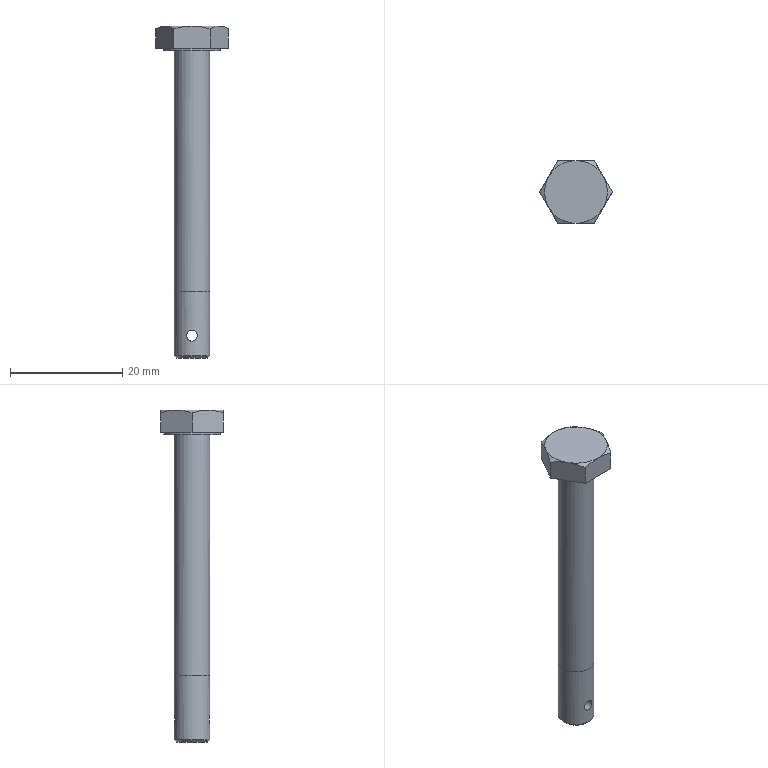Part | NX | features solid 2 | 1 solid | 21 faces | box 12.905 x 11.176 x 59.138 mm | volume 2174 mm3 | plane 10 | cone 7 | cylinder 4 | commonest cylinder face diameters 6.35 x2 1.93 x1 10.109 x1
STEP:
#1=CARTESIAN_POINT('',(0.,-3.175,-56.134));
#2=VERTEX_POINT('',#1);
#3=CARTESIAN_POINT('',(0.7569,-3.102,-55.925));
#4=CARTESIAN_POINT('',(-0.00006064,-3.212,-56.239));
#5=CARTESIAN_POINT('',(-0.7566,-3.102,-55.924));
#6=CARTESIAN_POINT('',(-1.07,-2.986,-55.17));
#7=CARTESIAN_POINT('',(-0.7562,-3.102,-54.412));
#8=CARTESIAN_POINT('',(-0.0005897,-3.212,-54.099));
#9=CARTESIAN_POINT('',(0.7561,-3.102,-54.412));
#10=CARTESIAN_POINT('',(1.07,-2.986,-55.169));
#11=CARTESIAN_POINT('',(0.7569,-3.102,-55.925));
#12=CARTESIAN_POINT('',(-0.00006064,-3.212,-56.239));
#13=CARTESIAN_POINT('',(-0.7566,-3.102,-55.924));
#14=B_SPLINE_CURVE_WITH_KNOTS('',3,(#3,#4,#5,#6,#7,#8,#9,#10,#11,#12,#13),.UNSPECIFIED.,.T.,.F.,(1,1,1,1,1,1,1,1,1,1,1,1,1,1,1),(-0.002276,-0.001518,-0.0007588,0.,0.0007588,0.001518,0.002276,0.003035,0.003794,0.004553,0.005312,0.006071,0.006829,0.007588,0.008347),.UNSPECIFIED.);
#15=EDGE_CURVE('',#2,#2,#14,.T.);
#16=ORIENTED_EDGE('',*,*,#15,.T.);
#17=EDGE_LOOP('',(#16));
#18=FACE_BOUND('',#17,.T.);
#19=CARTESIAN_POINT('',(-3.175,0.,-47.231));
#20=VERTEX_POINT('',#19);
#21=CARTESIAN_POINT('',(-2.488,2.488,-47.231));
#22=CARTESIAN_POINT('',(-3.519,0.,-47.231));
#23=CARTESIAN_POINT('',(-2.488,-2.488,-47.231));
#24=CARTESIAN_POINT('',(0.,-3.519,-47.231));
#25=CARTESIAN_POINT('',(2.488,-2.488,-47.231));
#26=CARTESIAN_POINT('',(3.519,0.,-47.231));
#27=CARTESIAN_POINT('',(2.488,2.488,-47.231));
#28=CARTESIAN_POINT('',(0.,3.519,-47.231));
#29=CARTESIAN_POINT('',(-2.488,2.488,-47.231));
#30=CARTESIAN_POINT('',(-3.519,0.,-47.231));
#31=CARTESIAN_POINT('',(-2.488,-2.488,-47.231));
#32=B_SPLINE_CURVE_WITH_KNOTS('',3,(#21,#22,#23,#24,#25,#26,#27,#28,#29,#30,#31),.UNSPECIFIED.,.T.,.F.,(1,1,1,1,1,1,1,1,1,1,1,1,1,1,1),(-0.375,-0.25,-0.125,0.,0.125,0.25,0.375,0.5,0.625,0.75,0.875,1.,1.125,1.25,1.375),.UNSPECIFIED.);
#33=EDGE_CURVE('',#20,#20,#32,.T.);
#34=ORIENTED_EDGE('',*,*,#33,.F.);
#35=EDGE_LOOP('',(#34));
#36=FACE_BOUND('',#35,.T.);
#37=CARTESIAN_POINT('',(-3.175,0.,-58.757));
#38=VERTEX_POINT('',#37);
#39=CARTESIAN_POINT('',(0.,0.,-58.757));
#40=DIRECTION('',(0.,0.,-1.));
#41=DIRECTION('',(-1.,0.,0.));
#42=AXIS2_PLACEMENT_3D('',#39,#40,#41);
#43=CIRCLE('',#42,3.175);
#44=EDGE_CURVE('',#38,#38,#43,.T.);
#45=ORIENTED_EDGE('',*,*,#44,.F.);
#46=EDGE_LOOP('',(#45));
#47=FACE_BOUND('',#46,.T.);
#48=CARTESIAN_POINT('',(0.,3.175,-56.134));
#49=VERTEX_POINT('',#48);
#50=CARTESIAN_POINT('',(-0.7569,3.102,-55.925));
#51=CARTESIAN_POINT('',(0.00006064,3.212,-56.239));
#52=CARTESIAN_POINT('',(0.7566,3.102,-55.924));
#53=CARTESIAN_POINT('',(1.07,2.986,-55.17));
#54=CARTESIAN_POINT('',(0.7562,3.102,-54.412));
#55=CARTESIAN_POINT('',(0.0005897,3.212,-54.099));
#56=CARTESIAN_POINT('',(-0.7561,3.102,-54.412));
#57=CARTESIAN_POINT('',(-1.07,2.986,-55.169));
#58=CARTESIAN_POINT('',(-0.7569,3.102,-55.925));
#59=CARTESIAN_POINT('',(0.00006064,3.212,-56.239));
#60=CARTESIAN_POINT('',(0.7566,3.102,-55.924));
#61=B_SPLINE_CURVE_WITH_KNOTS('',3,(#50,#51,#52,#53,#54,#55,#56,#57,#58,#59,#60),.UNSPECIFIED.,.T.,.F.,(1,1,1,1,1,1,1,1,1,1,1,1,1,1,1),(-0.002276,-0.001518,-0.0007588,0.,0.0007588,0.001518,0.002276,0.003035,0.003794,0.004553,0.005312,0.006071,0.006829,0.007588,0.008347),.UNSPECIFIED.);
#62=EDGE_CURVE('',#49,#49,#61,.T.);
#63=ORIENTED_EDGE('',*,*,#62,.T.);
#64=EDGE_LOOP('',(#63));
#65=FACE_BOUND('',#64,.T.);
#66=CARTESIAN_POINT('',(0.,0.,0.));
#67=DIRECTION('',(0.,0.,-1.));
#68=DIRECTION('',(-1.,0.,0.));
#69=AXIS2_PLACEMENT_3D('',#66,#67,#68);
#70=CYLINDRICAL_SURFACE('',#69,3.175);
#71=ADVANCED_FACE('',(#18,#36,#47,#65),#70,.T.);
#72=CARTESIAN_POINT('',(-3.175,0.,-4.369));
#73=VERTEX_POINT('',#72);
#74=CARTESIAN_POINT('',(0.,0.,-4.369));
#75=DIRECTION('',(0.,0.,-1.));
#76=DIRECTION('',(-1.,0.,0.));
#77=AXIS2_PLACEMENT_3D('',#74,#75,#76);
#78=CIRCLE('',#77,3.175);
#79=EDGE_CURVE('',#73,#73,#78,.T.);
#80=ORIENTED_EDGE('',*,*,#79,.T.);
#81=EDGE_LOOP('',(#80));
#82=FACE_BOUND('',#81,.T.);
#83=ORIENTED_EDGE('',*,*,#33,.T.);
#84=EDGE_LOOP('',(#83));
#85=FACE_BOUND('',#84,.T.);
#86=CARTESIAN_POINT('',(0.,0.,0.));
#87=DIRECTION('',(0.,0.,-1.));
#88=DIRECTION('',(-1.,0.,0.));
#89=AXIS2_PLACEMENT_3D('',#86,#87,#88);
#90=CYLINDRICAL_SURFACE('',#89,3.175);
#91=ADVANCED_FACE('',(#82,#85),#90,.T.);
#92=CARTESIAN_POINT('',(-6.452,0.,-3.962));
#93=VERTEX_POINT('',#92);
#94=CARTESIAN_POINT('',(-3.226,5.588,-3.962));
#95=VERTEX_POINT('',#94);
#96=CARTESIAN_POINT('',(-3.576,4.983,-3.962));
#97=DIRECTION('',(0.5,0.866,0.));
#98=VECTOR('',#97,1000.);
#99=LINE('',#96,#98);
#100=EDGE_CURVE('',#93,#95,#99,.T.);
#101=ORIENTED_EDGE('',*,*,#100,.T.);
#102=CARTESIAN_POINT('',(3.226,5.588,-3.962));
#103=VERTEX_POINT('',#102);
#104=CARTESIAN_POINT('',(5.055,5.588,-3.962));
#105=DIRECTION('',(1.,0.,0.));
#106=VECTOR('',#105,1000.);
#107=LINE('',#104,#106);
#108=EDGE_CURVE('',#95,#103,#107,.T.);
#109=ORIENTED_EDGE('',*,*,#108,.T.);
#110=CARTESIAN_POINT('',(6.452,0.,-3.962));
#111=VERTEX_POINT('',#110);
#112=CARTESIAN_POINT('',(6.103,0.6053,-3.962));
#113=DIRECTION('',(0.5,-0.866,0.));
#114=VECTOR('',#113,1000.);
#115=LINE('',#112,#114);
#116=EDGE_CURVE('',#103,#111,#115,.T.);
#117=ORIENTED_EDGE('',*,*,#116,.T.);
#118=CARTESIAN_POINT('',(3.226,-5.588,-3.962));
#119=VERTEX_POINT('',#118);
#120=CARTESIAN_POINT('',(6.103,-0.6053,-3.962));
#121=DIRECTION('',(-0.5,-0.866,0.));
#122=VECTOR('',#121,1000.);
#123=LINE('',#120,#122);
#124=EDGE_CURVE('',#111,#119,#123,.T.);
#125=ORIENTED_EDGE('',*,*,#124,.T.);
#126=CARTESIAN_POINT('',(-3.226,-5.588,-3.962));
#127=VERTEX_POINT('',#126);
#128=CARTESIAN_POINT('',(5.055,-5.588,-3.962));
#129=DIRECTION('',(-1.,0.,0.));
#130=VECTOR('',#129,1000.);
#131=LINE('',#128,#130);
#132=EDGE_CURVE('',#119,#127,#131,.T.);
#133=ORIENTED_EDGE('',*,*,#132,.T.);
#134=CARTESIAN_POINT('',(-3.576,-4.983,-3.962));
#135=DIRECTION('',(-0.5,0.866,0.));
#136=VECTOR('',#135,1000.);
#137=LINE('',#134,#136);
#138=EDGE_CURVE('',#127,#93,#137,.T.);
#139=ORIENTED_EDGE('',*,*,#138,.T.);
#140=EDGE_LOOP('',(#101,#109,#117,#125,#133,#139));
#141=FACE_BOUND('',#140,.T.);
#142=CARTESIAN_POINT('',(-5.055,0.,-3.962));
#143=VERTEX_POINT('',#142);
#144=CARTESIAN_POINT('',(0.,0.,-3.962));
#145=DIRECTION('',(0.,0.,-1.));
#146=DIRECTION('',(-1.,0.,0.));
#147=AXIS2_PLACEMENT_3D('',#144,#145,#146);
#148=CIRCLE('',#147,5.055);
#149=EDGE_CURVE('',#143,#143,#148,.T.);
#150=ORIENTED_EDGE('',*,*,#149,.F.);
#151=EDGE_LOOP('',(#150));
#152=FACE_BOUND('',#151,.T.);
#153=CARTESIAN_POINT('',(5.055,0.,-3.962));
#154=DIRECTION('',(0.,0.,-1.));
#155=DIRECTION('',(-1.,0.,0.));
#156=AXIS2_PLACEMENT_3D('',#153,#154,#155);
#157=PLANE('',#156);
#158=ADVANCED_FACE('',(#141,#152),#157,.T.);
#159=CARTESIAN_POINT('',(-2.794,0.,-59.138));
#160=VERTEX_POINT('',#159);
#161=CARTESIAN_POINT('',(0.,0.,-59.138));
#162=DIRECTION('',(0.,0.,-1.));
#163=DIRECTION('',(-1.,0.,0.));
#164=AXIS2_PLACEMENT_3D('',#161,#162,#163);
#165=CIRCLE('',#164,2.794);
#166=EDGE_CURVE('',#160,#160,#165,.T.);
#167=ORIENTED_EDGE('',*,*,#166,.T.);
#168=EDGE_LOOP('',(#167));
#169=FACE_BOUND('',#168,.T.);
#170=CARTESIAN_POINT('',(0.,0.,-59.138));
#171=DIRECTION('',(0.,0.,-1.));
#172=DIRECTION('',(-1.,0.,0.));
#173=AXIS2_PLACEMENT_3D('',#170,#171,#172);
#174=PLANE('',#173);
#175=ADVANCED_FACE('',(#169),#174,.T.);
#176=ORIENTED_EDGE('',*,*,#44,.T.);
#177=EDGE_LOOP('',(#176));
#178=FACE_BOUND('',#177,.T.);
#179=ORIENTED_EDGE('',*,*,#166,.F.);
#180=EDGE_LOOP('',(#179));
#181=FACE_BOUND('',#180,.T.);
#182=CARTESIAN_POINT('',(0.,0.,-59.138));
#183=DIRECTION('',(0.,0.,1.));
#184=DIRECTION('',(1.,0.,0.));
#185=AXIS2_PLACEMENT_3D('',#182,#183,#184);
#186=CONICAL_SURFACE('',#185,2.794,0.7854);
#187=ADVANCED_FACE('',(#178,#181),#186,.T.);
#188=CARTESIAN_POINT('',(-5.055,0.,-4.369));
#189=VERTEX_POINT('',#188);
#190=CARTESIAN_POINT('',(0.,0.,-4.369));
#191=DIRECTION('',(0.,0.,-1.));
#192=DIRECTION('',(-1.,0.,0.));
#193=AXIS2_PLACEMENT_3D('',#190,#191,#192);
#194=CIRCLE('',#193,5.055);
#195=EDGE_CURVE('',#189,#189,#194,.T.);
#196=ORIENTED_EDGE('',*,*,#195,.T.);
#197=EDGE_LOOP('',(#196));
#198=FACE_BOUND('',#197,.T.);
#199=ORIENTED_EDGE('',*,*,#79,.F.);
#200=EDGE_LOOP('',(#199));
#201=FACE_BOUND('',#200,.T.);
#202=CARTESIAN_POINT('',(3.175,0.,-4.369));
#203=DIRECTION('',(0.,0.,-1.));
#204=DIRECTION('',(-1.,0.,0.));
#205=AXIS2_PLACEMENT_3D('',#202,#203,#204);
#206=PLANE('',#205);
#207=ADVANCED_FACE('',(#198,#201),#206,.T.);
#208=ORIENTED_EDGE('',*,*,#149,.T.);
#209=EDGE_LOOP('',(#208));
#210=FACE_BOUND('',#209,.T.);
#211=ORIENTED_EDGE('',*,*,#195,.F.);
#212=EDGE_LOOP('',(#211));
#213=FACE_BOUND('',#212,.T.);
#214=CARTESIAN_POINT('',(0.,0.,0.));
#215=DIRECTION('',(0.,0.,-1.));
#216=DIRECTION('',(-1.,0.,0.));
#217=AXIS2_PLACEMENT_3D('',#214,#215,#216);
#218=CYLINDRICAL_SURFACE('',#217,5.055);
#219=ADVANCED_FACE('',(#210,#213),#218,.T.);
#220=ORIENTED_EDGE('',*,*,#108,.F.);
#221=CARTESIAN_POINT('',(-3.226,5.588,-0.4991));
#222=VERTEX_POINT('',#221);
#223=CARTESIAN_POINT('',(-3.226,5.588,-65.051));
#224=DIRECTION('',(0.,0.,1.));
#225=VECTOR('',#224,1000.);
#226=LINE('',#223,#225);
#227=EDGE_CURVE('',#95,#222,#226,.T.);
#228=ORIENTED_EDGE('',*,*,#227,.T.);
#229=CARTESIAN_POINT('',(0.,5.588,0.));
#230=VERTEX_POINT('',#229);
#231=CARTESIAN_POINT('',(-3.226,5.588,-0.4991));
#232=CARTESIAN_POINT('',(-2.177,5.588,-0.1961));
#233=CARTESIAN_POINT('',(-1.09,5.588,0.));
#234=CARTESIAN_POINT('',(0.,5.588,0.));
#235=B_SPLINE_CURVE_WITH_KNOTS('',3,(#231,#232,#233,#234),.UNSPECIFIED.,.F.,.F.,(4,4),(0.005758,0.009022),.UNSPECIFIED.);
#236=EDGE_CURVE('',#230,#222,#235,.F.);
#237=ORIENTED_EDGE('',*,*,#236,.F.);
#238=CARTESIAN_POINT('',(3.226,5.588,-0.4991));
#239=VERTEX_POINT('',#238);
#240=CARTESIAN_POINT('',(0.,5.588,0.));
#241=CARTESIAN_POINT('',(1.091,5.588,0.));
#242=CARTESIAN_POINT('',(2.183,5.588,-0.1979));
#243=CARTESIAN_POINT('',(3.226,5.588,-0.4991));
#244=B_SPLINE_CURVE_WITH_KNOTS('',3,(#240,#241,#242,#243),.UNSPECIFIED.,.F.,.F.,(4,4),(0.009022,0.01229),.UNSPECIFIED.);
#245=EDGE_CURVE('',#239,#230,#244,.F.);
#246=ORIENTED_EDGE('',*,*,#245,.F.);
#247=CARTESIAN_POINT('',(3.226,5.588,-65.051));
#248=DIRECTION('',(0.,0.,1.));
#249=VECTOR('',#248,1000.);
#250=LINE('',#247,#249);
#251=EDGE_CURVE('',#103,#239,#250,.T.);
#252=ORIENTED_EDGE('',*,*,#251,.F.);
#253=EDGE_LOOP('',(#220,#228,#237,#246,#252));
#254=FACE_BOUND('',#253,.T.);
#255=CARTESIAN_POINT('',(3.226,5.588,-65.051));
#256=DIRECTION('',(0.,1.,0.));
#257=DIRECTION('',(0.,0.,1.));
#258=AXIS2_PLACEMENT_3D('',#255,#256,#257);
#259=PLANE('',#258);
#260=ADVANCED_FACE('',(#254),#259,.T.);
#261=ORIENTED_EDGE('',*,*,#100,.F.);
#262=CARTESIAN_POINT('',(-6.452,0.,-0.4991));
#263=VERTEX_POINT('',#262);
#264=CARTESIAN_POINT('',(-6.452,0.,-65.051));
#265=DIRECTION('',(0.,0.,1.));
#266=VECTOR('',#265,1000.);
#267=LINE('',#264,#266);
#268=EDGE_CURVE('',#93,#263,#267,.T.);
#269=ORIENTED_EDGE('',*,*,#268,.T.);
#270=CARTESIAN_POINT('',(-4.839,2.794,0.));
#271=VERTEX_POINT('',#270);
#272=CARTESIAN_POINT('',(-4.839,2.794,0.));
#273=CARTESIAN_POINT('',(-5.387,1.846,0.));
#274=CARTESIAN_POINT('',(-5.926,0.9118,-0.1952));
#275=CARTESIAN_POINT('',(-6.452,0.,-0.4991));
#276=B_SPLINE_CURVE_WITH_KNOTS('',3,(#272,#273,#274,#275),.UNSPECIFIED.,.F.,.F.,(4,4),(0.003265,0.006517),.UNSPECIFIED.);
#277=EDGE_CURVE('',#271,#263,#276,.T.);
#278=ORIENTED_EDGE('',*,*,#277,.F.);
#279=CARTESIAN_POINT('',(-3.226,5.588,-0.4991));
#280=CARTESIAN_POINT('',(-3.754,4.674,-0.1944));
#281=CARTESIAN_POINT('',(-4.29,3.746,0.));
#282=CARTESIAN_POINT('',(-4.839,2.794,0.));
#283=B_SPLINE_CURVE_WITH_KNOTS('',3,(#279,#280,#281,#282),.UNSPECIFIED.,.F.,.F.,(4,4),(0.000000238,0.003265),.UNSPECIFIED.);
#284=EDGE_CURVE('',#222,#271,#283,.T.);
#285=ORIENTED_EDGE('',*,*,#284,.F.);
#286=ORIENTED_EDGE('',*,*,#227,.F.);
#287=EDGE_LOOP('',(#261,#269,#278,#285,#286));
#288=FACE_BOUND('',#287,.T.);
#289=CARTESIAN_POINT('',(-3.226,5.588,-65.051));
#290=DIRECTION('',(-0.866,0.5,0.));
#291=DIRECTION('',(-0.5,-0.866,0.));
#292=AXIS2_PLACEMENT_3D('',#289,#290,#291);
#293=PLANE('',#292);
#294=ADVANCED_FACE('',(#288),#293,.T.);
#295=ORIENTED_EDGE('',*,*,#138,.F.);
#296=CARTESIAN_POINT('',(-3.226,-5.588,-0.4991));
#297=VERTEX_POINT('',#296);
#298=CARTESIAN_POINT('',(-3.226,-5.588,-65.051));
#299=DIRECTION('',(0.,0.,1.));
#300=VECTOR('',#299,1000.);
#301=LINE('',#298,#300);
#302=EDGE_CURVE('',#127,#297,#301,.T.);
#303=ORIENTED_EDGE('',*,*,#302,.T.);
#304=CARTESIAN_POINT('',(-4.839,-2.794,0.));
#305=VERTEX_POINT('',#304);
#306=CARTESIAN_POINT('',(-4.839,-2.794,0.));
#307=CARTESIAN_POINT('',(-4.292,-3.742,0.));
#308=CARTESIAN_POINT('',(-3.753,-4.676,-0.1952));
#309=CARTESIAN_POINT('',(-3.226,-5.588,-0.4991));
#310=B_SPLINE_CURVE_WITH_KNOTS('',3,(#306,#307,#308,#309),.UNSPECIFIED.,.F.,.F.,(4,4),(0.003265,0.006517),.UNSPECIFIED.);
#311=EDGE_CURVE('',#305,#297,#310,.T.);
#312=ORIENTED_EDGE('',*,*,#311,.F.);
#313=CARTESIAN_POINT('',(-6.452,0.,-0.4991));
#314=CARTESIAN_POINT('',(-5.925,-0.9141,-0.1944));
#315=CARTESIAN_POINT('',(-5.389,-1.842,0.));
#316=CARTESIAN_POINT('',(-4.839,-2.794,0.));
#317=B_SPLINE_CURVE_WITH_KNOTS('',3,(#313,#314,#315,#316),.UNSPECIFIED.,.F.,.F.,(4,4),(0.000000238,0.003265),.UNSPECIFIED.);
#318=EDGE_CURVE('',#263,#305,#317,.T.);
#319=ORIENTED_EDGE('',*,*,#318,.F.);
#320=ORIENTED_EDGE('',*,*,#268,.F.);
#321=EDGE_LOOP('',(#295,#303,#312,#319,#320));
#322=FACE_BOUND('',#321,.T.);
#323=CARTESIAN_POINT('',(-6.452,0.,-65.051));
#324=DIRECTION('',(-0.866,-0.5,0.));
#325=DIRECTION('',(0.5,-0.866,0.));
#326=AXIS2_PLACEMENT_3D('',#323,#324,#325);
#327=PLANE('',#326);
#328=ADVANCED_FACE('',(#322),#327,.T.);
#329=ORIENTED_EDGE('',*,*,#132,.F.);
#330=CARTESIAN_POINT('',(3.226,-5.588,-0.4991));
#331=VERTEX_POINT('',#330);
#332=CARTESIAN_POINT('',(3.226,-5.588,-65.051));
#333=DIRECTION('',(0.,0.,1.));
#334=VECTOR('',#333,1000.);
#335=LINE('',#332,#334);
#336=EDGE_CURVE('',#119,#331,#335,.T.);
#337=ORIENTED_EDGE('',*,*,#336,.T.);
#338=CARTESIAN_POINT('',(0.,-5.588,0.));
#339=VERTEX_POINT('',#338);
#340=CARTESIAN_POINT('',(0.,-5.588,0.));
#341=CARTESIAN_POINT('',(1.091,-5.588,0.));
#342=CARTESIAN_POINT('',(2.183,-5.588,-0.1979));
#343=CARTESIAN_POINT('',(3.226,-5.588,-0.4991));
#344=B_SPLINE_CURVE_WITH_KNOTS('',3,(#340,#341,#342,#343),.UNSPECIFIED.,.F.,.F.,(4,4),(0.009022,0.01229),.UNSPECIFIED.);
#345=EDGE_CURVE('',#339,#331,#344,.T.);
#346=ORIENTED_EDGE('',*,*,#345,.F.);
#347=CARTESIAN_POINT('',(-3.226,-5.588,-0.4991));
#348=CARTESIAN_POINT('',(-2.177,-5.588,-0.1961));
#349=CARTESIAN_POINT('',(-1.09,-5.588,0.));
#350=CARTESIAN_POINT('',(0.,-5.588,0.));
#351=B_SPLINE_CURVE_WITH_KNOTS('',3,(#347,#348,#349,#350),.UNSPECIFIED.,.F.,.F.,(4,4),(0.005758,0.009022),.UNSPECIFIED.);
#352=EDGE_CURVE('',#297,#339,#351,.T.);
#353=ORIENTED_EDGE('',*,*,#352,.F.);
#354=ORIENTED_EDGE('',*,*,#302,.F.);
#355=EDGE_LOOP('',(#329,#337,#346,#353,#354));
#356=FACE_BOUND('',#355,.T.);
#357=CARTESIAN_POINT('',(-3.226,-5.588,-65.051));
#358=DIRECTION('',(0.,-1.,0.));
#359=DIRECTION('',(0.,0.,-1.));
#360=AXIS2_PLACEMENT_3D('',#357,#358,#359);
#361=PLANE('',#360);
#362=ADVANCED_FACE('',(#356),#361,.T.);
#363=ORIENTED_EDGE('',*,*,#124,.F.);
#364=CARTESIAN_POINT('',(6.452,0.,-0.4991));
#365=VERTEX_POINT('',#364);
#366=CARTESIAN_POINT('',(6.452,0.,-65.051));
#367=DIRECTION('',(0.,0.,1.));
#368=VECTOR('',#367,1000.);
#369=LINE('',#366,#368);
#370=EDGE_CURVE('',#111,#365,#369,.T.);
#371=ORIENTED_EDGE('',*,*,#370,.T.);
#372=CARTESIAN_POINT('',(4.839,-2.794,0.));
#373=VERTEX_POINT('',#372);
#374=CARTESIAN_POINT('',(4.839,-2.794,0.));
#375=CARTESIAN_POINT('',(5.387,-1.846,0.));
#376=CARTESIAN_POINT('',(5.926,-0.9118,-0.1952));
#377=CARTESIAN_POINT('',(6.452,0.,-0.4991));
#378=B_SPLINE_CURVE_WITH_KNOTS('',3,(#374,#375,#376,#377),.UNSPECIFIED.,.F.,.F.,(4,4),(0.003265,0.006517),.UNSPECIFIED.);
#379=EDGE_CURVE('',#373,#365,#378,.T.);
#380=ORIENTED_EDGE('',*,*,#379,.F.);
#381=CARTESIAN_POINT('',(3.226,-5.588,-0.4991));
#382=CARTESIAN_POINT('',(3.754,-4.674,-0.1944));
#383=CARTESIAN_POINT('',(4.29,-3.746,0.));
#384=CARTESIAN_POINT('',(4.839,-2.794,0.));
#385=B_SPLINE_CURVE_WITH_KNOTS('',3,(#381,#382,#383,#384),.UNSPECIFIED.,.F.,.F.,(4,4),(0.000000238,0.003265),.UNSPECIFIED.);
#386=EDGE_CURVE('',#331,#373,#385,.T.);
#387=ORIENTED_EDGE('',*,*,#386,.F.);
#388=ORIENTED_EDGE('',*,*,#336,.F.);
#389=EDGE_LOOP('',(#363,#371,#380,#387,#388));
#390=FACE_BOUND('',#389,.T.);
#391=CARTESIAN_POINT('',(3.226,-5.588,-65.051));
#392=DIRECTION('',(0.866,-0.5,0.));
#393=DIRECTION('',(0.5,0.866,0.));
#394=AXIS2_PLACEMENT_3D('',#391,#392,#393);
#395=PLANE('',#394);
#396=ADVANCED_FACE('',(#390),#395,.T.);
#397=ORIENTED_EDGE('',*,*,#116,.F.);
#398=ORIENTED_EDGE('',*,*,#251,.T.);
#399=CARTESIAN_POINT('',(4.839,2.794,0.));
#400=VERTEX_POINT('',#399);
#401=CARTESIAN_POINT('',(4.839,2.794,0.));
#402=CARTESIAN_POINT('',(4.292,3.742,0.));
#403=CARTESIAN_POINT('',(3.753,4.676,-0.1952));
#404=CARTESIAN_POINT('',(3.226,5.588,-0.4991));
#405=B_SPLINE_CURVE_WITH_KNOTS('',3,(#401,#402,#403,#404),.UNSPECIFIED.,.F.,.F.,(4,4),(0.003265,0.006517),.UNSPECIFIED.);
#406=EDGE_CURVE('',#400,#239,#405,.T.);
#407=ORIENTED_EDGE('',*,*,#406,.F.);
#408=CARTESIAN_POINT('',(6.452,0.,-0.4991));
#409=CARTESIAN_POINT('',(5.925,0.9141,-0.1944));
#410=CARTESIAN_POINT('',(5.389,1.842,0.));
#411=CARTESIAN_POINT('',(4.839,2.794,0.));
#412=B_SPLINE_CURVE_WITH_KNOTS('',3,(#408,#409,#410,#411),.UNSPECIFIED.,.F.,.F.,(4,4),(0.000000238,0.003265),.UNSPECIFIED.);
#413=EDGE_CURVE('',#365,#400,#412,.T.);
#414=ORIENTED_EDGE('',*,*,#413,.F.);
#415=ORIENTED_EDGE('',*,*,#370,.F.);
#416=EDGE_LOOP('',(#397,#398,#407,#414,#415));
#417=FACE_BOUND('',#416,.T.);
#418=CARTESIAN_POINT('',(6.452,0.,-65.051));
#419=DIRECTION('',(0.866,0.5,0.));
#420=DIRECTION('',(-0.5,0.866,0.));
#421=AXIS2_PLACEMENT_3D('',#418,#419,#420);
#422=PLANE('',#421);
#423=ADVANCED_FACE('',(#417),#422,.T.);
#424=CARTESIAN_POINT('',(0.,0.,0.));
#425=DIRECTION('',(0.,0.,-1.));
#426=DIRECTION('',(-1.,0.,0.));
#427=AXIS2_PLACEMENT_3D('',#424,#425,#426);
#428=CIRCLE('',#427,5.588);
#429=EDGE_CURVE('',#400,#373,#428,.T.);
#430=ORIENTED_EDGE('',*,*,#429,.T.);
#431=ORIENTED_EDGE('',*,*,#379,.T.);
#432=ORIENTED_EDGE('',*,*,#413,.T.);
#433=EDGE_LOOP('',(#430,#431,#432));
#434=FACE_BOUND('',#433,.T.);
#435=CARTESIAN_POINT('',(0.,0.,-0.5133));
#436=DIRECTION('',(0.,0.,-1.));
#437=DIRECTION('',(-1.,0.,0.));
#438=AXIS2_PLACEMENT_3D('',#435,#436,#437);
#439=CONICAL_SURFACE('',#438,6.477,1.047);
#440=ADVANCED_FACE('',(#434),#439,.T.);
#441=CARTESIAN_POINT('',(0.,0.,0.));
#442=DIRECTION('',(0.,0.,-1.));
#443=DIRECTION('',(-1.,0.,0.));
#444=AXIS2_PLACEMENT_3D('',#441,#442,#443);
#445=CIRCLE('',#444,5.588);
#446=EDGE_CURVE('',#373,#339,#445,.T.);
#447=ORIENTED_EDGE('',*,*,#446,.T.);
#448=ORIENTED_EDGE('',*,*,#345,.T.);
#449=ORIENTED_EDGE('',*,*,#386,.T.);
#450=EDGE_LOOP('',(#447,#448,#449));
#451=FACE_BOUND('',#450,.T.);
#452=CARTESIAN_POINT('',(0.,0.,-0.5133));
#453=DIRECTION('',(0.,0.,-1.));
#454=DIRECTION('',(-1.,0.,0.));
#455=AXIS2_PLACEMENT_3D('',#452,#453,#454);
#456=CONICAL_SURFACE('',#455,6.477,1.047);
#457=ADVANCED_FACE('',(#451),#456,.T.);
#458=CARTESIAN_POINT('',(0.,0.,0.));
#459=DIRECTION('',(0.,0.,-1.));
#460=DIRECTION('',(-1.,0.,0.));
#461=AXIS2_PLACEMENT_3D('',#458,#459,#460);
#462=CIRCLE('',#461,5.588);
#463=EDGE_CURVE('',#339,#305,#462,.T.);
#464=ORIENTED_EDGE('',*,*,#463,.T.);
#465=ORIENTED_EDGE('',*,*,#311,.T.);
#466=ORIENTED_EDGE('',*,*,#352,.T.);
#467=EDGE_LOOP('',(#464,#465,#466));
#468=FACE_BOUND('',#467,.T.);
#469=CARTESIAN_POINT('',(0.,0.,-0.5133));
#470=DIRECTION('',(0.,0.,-1.));
#471=DIRECTION('',(-1.,0.,0.));
#472=AXIS2_PLACEMENT_3D('',#469,#470,#471);
#473=CONICAL_SURFACE('',#472,6.477,1.047);
#474=ADVANCED_FACE('',(#468),#473,.T.);
#475=CARTESIAN_POINT('',(0.,0.,0.));
#476=DIRECTION('',(0.,0.,-1.));
#477=DIRECTION('',(-1.,0.,0.));
#478=AXIS2_PLACEMENT_3D('',#475,#476,#477);
#479=CIRCLE('',#478,5.588);
#480=EDGE_CURVE('',#305,#271,#479,.T.);
#481=ORIENTED_EDGE('',*,*,#480,.T.);
#482=ORIENTED_EDGE('',*,*,#277,.T.);
#483=ORIENTED_EDGE('',*,*,#318,.T.);
#484=EDGE_LOOP('',(#481,#482,#483));
#485=FACE_BOUND('',#484,.T.);
#486=CARTESIAN_POINT('',(0.,0.,-0.5133));
#487=DIRECTION('',(0.,0.,-1.));
#488=DIRECTION('',(-1.,0.,0.));
#489=AXIS2_PLACEMENT_3D('',#486,#487,#488);
#490=CONICAL_SURFACE('',#489,6.477,1.047);
#491=ADVANCED_FACE('',(#485),#490,.T.);
#492=CARTESIAN_POINT('',(0.,0.,0.));
#493=DIRECTION('',(0.,0.,-1.));
#494=DIRECTION('',(-1.,0.,0.));
#495=AXIS2_PLACEMENT_3D('',#492,#493,#494);
#496=CIRCLE('',#495,5.588);
#497=EDGE_CURVE('',#271,#230,#496,.T.);
#498=ORIENTED_EDGE('',*,*,#497,.T.);
#499=ORIENTED_EDGE('',*,*,#236,.T.);
#500=ORIENTED_EDGE('',*,*,#284,.T.);
#501=EDGE_LOOP('',(#498,#499,#500));
#502=FACE_BOUND('',#501,.T.);
#503=CARTESIAN_POINT('',(0.,0.,-0.5133));
#504=DIRECTION('',(0.,0.,-1.));
#505=DIRECTION('',(-1.,0.,0.));
#506=AXIS2_PLACEMENT_3D('',#503,#504,#505);
#507=CONICAL_SURFACE('',#506,6.477,1.047);
#508=ADVANCED_FACE('',(#502),#507,.T.);
#509=ORIENTED_EDGE('',*,*,#497,.F.);
#510=ORIENTED_EDGE('',*,*,#480,.F.);
#511=ORIENTED_EDGE('',*,*,#463,.F.);
#512=ORIENTED_EDGE('',*,*,#446,.F.);
#513=ORIENTED_EDGE('',*,*,#429,.F.);
#514=CARTESIAN_POINT('',(0.,0.,0.));
#515=DIRECTION('',(0.,0.,-1.));
#516=DIRECTION('',(-1.,0.,0.));
#517=AXIS2_PLACEMENT_3D('',#514,#515,#516);
#518=CIRCLE('',#517,5.588);
#519=EDGE_CURVE('',#230,#400,#518,.T.);
#520=ORIENTED_EDGE('',*,*,#519,.F.);
#521=EDGE_LOOP('',(#509,#510,#511,#512,#513,#520));
#522=FACE_BOUND('',#521,.T.);
#523=CARTESIAN_POINT('',(5.588,0.,0.));
#524=DIRECTION('',(0.,0.,1.));
#525=DIRECTION('',(1.,0.,0.));
#526=AXIS2_PLACEMENT_3D('',#523,#524,#525);
#527=PLANE('',#526);
#528=ADVANCED_FACE('',(#522),#527,.T.);
#529=ORIENTED_EDGE('',*,*,#406,.T.);
#530=ORIENTED_EDGE('',*,*,#245,.T.);
#531=ORIENTED_EDGE('',*,*,#519,.T.);
#532=EDGE_LOOP('',(#529,#530,#531));
#533=FACE_BOUND('',#532,.T.);
#534=CARTESIAN_POINT('',(0.,0.,-0.5133));
#535=DIRECTION('',(0.,0.,-1.));
#536=DIRECTION('',(-1.,0.,0.));
#537=AXIS2_PLACEMENT_3D('',#534,#535,#536);
#538=CONICAL_SURFACE('',#537,6.477,1.047);
#539=ADVANCED_FACE('',(#533),#538,.T.);
#540=ORIENTED_EDGE('',*,*,#62,.F.);
#541=EDGE_LOOP('',(#540));
#542=FACE_BOUND('',#541,.T.);
#543=ORIENTED_EDGE('',*,*,#15,.F.);
#544=EDGE_LOOP('',(#543));
#545=FACE_BOUND('',#544,.T.);
#546=CARTESIAN_POINT('',(0.,6.147,-55.169));
#547=DIRECTION('',(0.,-1.,0.));
#548=DIRECTION('',(0.,0.,-1.));
#549=AXIS2_PLACEMENT_3D('',#546,#547,#548);
#550=CYLINDRICAL_SURFACE('',#549,0.9652);
#551=ADVANCED_FACE('',(#542,#545),#550,.F.);
#552=CLOSED_SHELL('',(#71,#91,#158,#175,#187,#207,#219,#260,#294,#328,#362,#396,#423,#440,#457,#474,#491,#508,#528,#539,#551));
#553=MANIFOLD_SOLID_BREP('',#552);
#554=(LENGTH_UNIT()NAMED_UNIT(*)SI_UNIT(.MILLI.,.METRE.));
#555=UNCERTAINTY_MEASURE_WITH_UNIT(LENGTH_MEASURE(0.0508),#554,'','');
#556=(NAMED_UNIT(*)PLANE_ANGLE_UNIT()SI_UNIT($,.RADIAN.));
#557=(NAMED_UNIT(*)SI_UNIT($,.STERADIAN.)SOLID_ANGLE_UNIT());
#558=(GEOMETRIC_REPRESENTATION_CONTEXT(3)GLOBAL_UNCERTAINTY_ASSIGNED_CONTEXT((#555))GLOBAL_UNIT_ASSIGNED_CONTEXT((#554,#556,#557))REPRESENTATION_CONTEXT('',''));
#559=ADVANCED_BREP_SHAPE_REPRESENTATION('',(#553),#558);